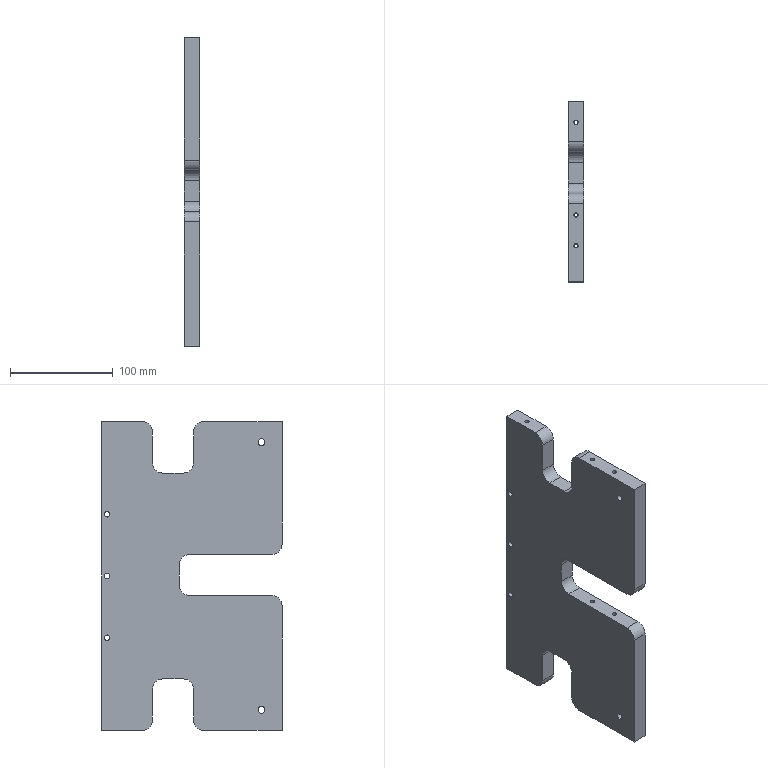Part | SolidWorks | features HoleWzd 10, MirrorPattern 9, LPattern 6, Cut 4, ICE 3, Fillet 2, Extrusion 1 | 1 solid | 267 faces | box 15 x 175 x 300 mm | volume 650278 mm3 | cylinder 139 | plane 102 | cone 26 | commonest cylinder face diameters 4 x44 2.5 x24 4.2 x20 2 x13 20 x12 3.3 x6